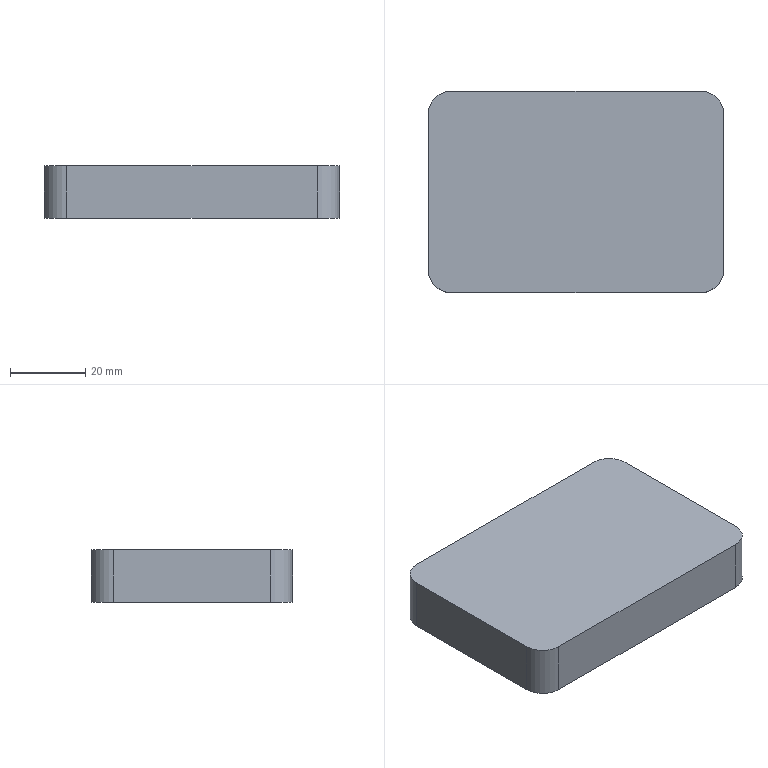Part | SolidWorks | features Extrusion 1, Fillet 1 | 1 solid | 10 faces | box 78.5 x 53.5 x 14 mm | volume 58364 mm3 | plane 6 | cylinder 4 | commonest cylinder face diameters 12 x4
STEP:
#1=CARTESIAN_POINT('',(0.,47.5,0.));
#2=VERTEX_POINT('',#1);
#3=CARTESIAN_POINT('',(0.,6.,0.));
#4=VERTEX_POINT('',#3);
#5=CARTESIAN_POINT('',(0.,0.,0.));
#6=DIRECTION('',(0.,-1.,0.));
#7=VECTOR('',#6,1000.);
#8=LINE('',#5,#7);
#9=EDGE_CURVE('',#2,#4,#8,.T.);
#10=ORIENTED_EDGE('',*,*,#9,.T.);
#11=CARTESIAN_POINT('',(0.,6.,14.));
#12=VERTEX_POINT('',#11);
#13=CARTESIAN_POINT('',(0.,6.,14.));
#14=DIRECTION('',(0.,0.,1.));
#15=VECTOR('',#14,1000.);
#16=LINE('',#13,#15);
#17=EDGE_CURVE('',#4,#12,#16,.T.);
#18=ORIENTED_EDGE('',*,*,#17,.T.);
#19=CARTESIAN_POINT('',(0.,47.5,14.));
#20=VERTEX_POINT('',#19);
#21=CARTESIAN_POINT('',(0.,0.,14.));
#22=DIRECTION('',(0.,-1.,0.));
#23=VECTOR('',#22,1000.);
#24=LINE('',#21,#23);
#25=EDGE_CURVE('',#20,#12,#24,.T.);
#26=ORIENTED_EDGE('',*,*,#25,.F.);
#27=CARTESIAN_POINT('',(0.,47.5,14.));
#28=DIRECTION('',(0.,0.,-1.));
#29=VECTOR('',#28,1000.);
#30=LINE('',#27,#29);
#31=EDGE_CURVE('',#20,#2,#30,.T.);
#32=ORIENTED_EDGE('',*,*,#31,.T.);
#33=EDGE_LOOP('',(#10,#18,#26,#32));
#34=FACE_OUTER_BOUND('',#33,.T.);
#35=CARTESIAN_POINT('',(0.,0.,14.));
#36=DIRECTION('',(1.,0.,0.));
#37=DIRECTION('',(0.,0.,-1.));
#38=AXIS2_PLACEMENT_3D('',#35,#36,#37);
#39=PLANE('',#38);
#40=ADVANCED_FACE('',(#34),#39,.F.);
#41=CARTESIAN_POINT('',(6.,0.,0.));
#42=VERTEX_POINT('',#41);
#43=CARTESIAN_POINT('',(72.5,0.,0.));
#44=VERTEX_POINT('',#43);
#45=CARTESIAN_POINT('',(0.,0.,0.));
#46=DIRECTION('',(1.,0.,0.));
#47=VECTOR('',#46,1000.);
#48=LINE('',#45,#47);
#49=EDGE_CURVE('',#42,#44,#48,.T.);
#50=ORIENTED_EDGE('',*,*,#49,.T.);
#51=CARTESIAN_POINT('',(72.5,0.,14.));
#52=VERTEX_POINT('',#51);
#53=CARTESIAN_POINT('',(72.5,0.,14.));
#54=DIRECTION('',(0.,0.,1.));
#55=VECTOR('',#54,1000.);
#56=LINE('',#53,#55);
#57=EDGE_CURVE('',#44,#52,#56,.T.);
#58=ORIENTED_EDGE('',*,*,#57,.T.);
#59=CARTESIAN_POINT('',(6.,0.,14.));
#60=VERTEX_POINT('',#59);
#61=CARTESIAN_POINT('',(0.,0.,14.));
#62=DIRECTION('',(1.,0.,0.));
#63=VECTOR('',#62,1000.);
#64=LINE('',#61,#63);
#65=EDGE_CURVE('',#60,#52,#64,.T.);
#66=ORIENTED_EDGE('',*,*,#65,.F.);
#67=CARTESIAN_POINT('',(6.,0.,14.));
#68=DIRECTION('',(0.,0.,-1.));
#69=VECTOR('',#68,1000.);
#70=LINE('',#67,#69);
#71=EDGE_CURVE('',#60,#42,#70,.T.);
#72=ORIENTED_EDGE('',*,*,#71,.T.);
#73=EDGE_LOOP('',(#50,#58,#66,#72));
#74=FACE_OUTER_BOUND('',#73,.T.);
#75=CARTESIAN_POINT('',(0.,0.,14.));
#76=DIRECTION('',(0.,1.,0.));
#77=DIRECTION('',(0.,0.,1.));
#78=AXIS2_PLACEMENT_3D('',#75,#76,#77);
#79=PLANE('',#78);
#80=ADVANCED_FACE('',(#74),#79,.F.);
#81=CARTESIAN_POINT('',(78.5,6.,0.));
#82=VERTEX_POINT('',#81);
#83=CARTESIAN_POINT('',(78.5,47.5,0.));
#84=VERTEX_POINT('',#83);
#85=CARTESIAN_POINT('',(78.5,0.,0.));
#86=DIRECTION('',(0.,1.,0.));
#87=VECTOR('',#86,1000.);
#88=LINE('',#85,#87);
#89=EDGE_CURVE('',#82,#84,#88,.T.);
#90=ORIENTED_EDGE('',*,*,#89,.T.);
#91=CARTESIAN_POINT('',(78.5,47.5,14.));
#92=VERTEX_POINT('',#91);
#93=CARTESIAN_POINT('',(78.5,47.5,14.));
#94=DIRECTION('',(0.,0.,1.));
#95=VECTOR('',#94,1000.);
#96=LINE('',#93,#95);
#97=EDGE_CURVE('',#84,#92,#96,.T.);
#98=ORIENTED_EDGE('',*,*,#97,.T.);
#99=CARTESIAN_POINT('',(78.5,6.,14.));
#100=VERTEX_POINT('',#99);
#101=CARTESIAN_POINT('',(78.5,0.,14.));
#102=DIRECTION('',(0.,1.,0.));
#103=VECTOR('',#102,1000.);
#104=LINE('',#101,#103);
#105=EDGE_CURVE('',#100,#92,#104,.T.);
#106=ORIENTED_EDGE('',*,*,#105,.F.);
#107=CARTESIAN_POINT('',(78.5,6.,14.));
#108=DIRECTION('',(0.,0.,-1.));
#109=VECTOR('',#108,1000.);
#110=LINE('',#107,#109);
#111=EDGE_CURVE('',#100,#82,#110,.T.);
#112=ORIENTED_EDGE('',*,*,#111,.T.);
#113=EDGE_LOOP('',(#90,#98,#106,#112));
#114=FACE_OUTER_BOUND('',#113,.T.);
#115=CARTESIAN_POINT('',(78.5,0.,14.));
#116=DIRECTION('',(-1.,0.,0.));
#117=DIRECTION('',(0.,0.,1.));
#118=AXIS2_PLACEMENT_3D('',#115,#116,#117);
#119=PLANE('',#118);
#120=ADVANCED_FACE('',(#114),#119,.F.);
#121=CARTESIAN_POINT('',(72.5,53.5,14.));
#122=VERTEX_POINT('',#121);
#123=CARTESIAN_POINT('',(6.,53.5,14.));
#124=VERTEX_POINT('',#123);
#125=CARTESIAN_POINT('',(0.,53.5,14.));
#126=DIRECTION('',(-1.,0.,0.));
#127=VECTOR('',#126,1000.);
#128=LINE('',#125,#127);
#129=EDGE_CURVE('',#122,#124,#128,.T.);
#130=ORIENTED_EDGE('',*,*,#129,.F.);
#131=CARTESIAN_POINT('',(72.5,53.5,0.));
#132=VERTEX_POINT('',#131);
#133=CARTESIAN_POINT('',(72.5,53.5,14.));
#134=DIRECTION('',(0.,0.,-1.));
#135=VECTOR('',#134,1000.);
#136=LINE('',#133,#135);
#137=EDGE_CURVE('',#122,#132,#136,.T.);
#138=ORIENTED_EDGE('',*,*,#137,.T.);
#139=CARTESIAN_POINT('',(6.,53.5,0.));
#140=VERTEX_POINT('',#139);
#141=CARTESIAN_POINT('',(0.,53.5,0.));
#142=DIRECTION('',(-1.,0.,0.));
#143=VECTOR('',#142,1000.);
#144=LINE('',#141,#143);
#145=EDGE_CURVE('',#132,#140,#144,.T.);
#146=ORIENTED_EDGE('',*,*,#145,.T.);
#147=CARTESIAN_POINT('',(6.,53.5,14.));
#148=DIRECTION('',(0.,0.,1.));
#149=VECTOR('',#148,1000.);
#150=LINE('',#147,#149);
#151=EDGE_CURVE('',#140,#124,#150,.T.);
#152=ORIENTED_EDGE('',*,*,#151,.T.);
#153=EDGE_LOOP('',(#130,#138,#146,#152));
#154=FACE_OUTER_BOUND('',#153,.T.);
#155=CARTESIAN_POINT('',(0.,53.5,14.));
#156=DIRECTION('',(0.,-1.,0.));
#157=DIRECTION('',(0.,0.,-1.));
#158=AXIS2_PLACEMENT_3D('',#155,#156,#157);
#159=PLANE('',#158);
#160=ADVANCED_FACE('',(#154),#159,.F.);
#161=ORIENTED_EDGE('',*,*,#105,.T.);
#162=CARTESIAN_POINT('',(72.5,47.5,14.));
#163=DIRECTION('',(0.,0.,1.));
#164=DIRECTION('',(-1.,0.,0.));
#165=AXIS2_PLACEMENT_3D('',#162,#163,#164);
#166=CIRCLE('',#165,6.);
#167=EDGE_CURVE('',#92,#122,#166,.T.);
#168=ORIENTED_EDGE('',*,*,#167,.T.);
#169=ORIENTED_EDGE('',*,*,#129,.T.);
#170=CARTESIAN_POINT('',(6.,47.5,14.));
#171=DIRECTION('',(0.,0.,1.));
#172=DIRECTION('',(-1.,0.,0.));
#173=AXIS2_PLACEMENT_3D('',#170,#171,#172);
#174=CIRCLE('',#173,6.);
#175=EDGE_CURVE('',#124,#20,#174,.T.);
#176=ORIENTED_EDGE('',*,*,#175,.T.);
#177=ORIENTED_EDGE('',*,*,#25,.T.);
#178=CARTESIAN_POINT('',(6.,6.,14.));
#179=DIRECTION('',(0.,0.,1.));
#180=DIRECTION('',(-1.,0.,0.));
#181=AXIS2_PLACEMENT_3D('',#178,#179,#180);
#182=CIRCLE('',#181,6.);
#183=EDGE_CURVE('',#12,#60,#182,.T.);
#184=ORIENTED_EDGE('',*,*,#183,.T.);
#185=ORIENTED_EDGE('',*,*,#65,.T.);
#186=CARTESIAN_POINT('',(72.5,6.,14.));
#187=DIRECTION('',(0.,0.,1.));
#188=DIRECTION('',(-1.,0.,0.));
#189=AXIS2_PLACEMENT_3D('',#186,#187,#188);
#190=CIRCLE('',#189,6.);
#191=EDGE_CURVE('',#52,#100,#190,.T.);
#192=ORIENTED_EDGE('',*,*,#191,.T.);
#193=EDGE_LOOP('',(#161,#168,#169,#176,#177,#184,#185,#192));
#194=FACE_OUTER_BOUND('',#193,.T.);
#195=CARTESIAN_POINT('',(0.,0.,14.));
#196=DIRECTION('',(0.,0.,-1.));
#197=DIRECTION('',(-1.,0.,0.));
#198=AXIS2_PLACEMENT_3D('',#195,#196,#197);
#199=PLANE('',#198);
#200=ADVANCED_FACE('',(#194),#199,.F.);
#201=ORIENTED_EDGE('',*,*,#145,.F.);
#202=CARTESIAN_POINT('',(72.5,47.5,0.));
#203=DIRECTION('',(0.,0.,-1.));
#204=DIRECTION('',(-1.,0.,0.));
#205=AXIS2_PLACEMENT_3D('',#202,#203,#204);
#206=CIRCLE('',#205,6.);
#207=EDGE_CURVE('',#132,#84,#206,.T.);
#208=ORIENTED_EDGE('',*,*,#207,.T.);
#209=ORIENTED_EDGE('',*,*,#89,.F.);
#210=CARTESIAN_POINT('',(72.5,6.,0.));
#211=DIRECTION('',(0.,0.,-1.));
#212=DIRECTION('',(-1.,0.,0.));
#213=AXIS2_PLACEMENT_3D('',#210,#211,#212);
#214=CIRCLE('',#213,6.);
#215=EDGE_CURVE('',#82,#44,#214,.T.);
#216=ORIENTED_EDGE('',*,*,#215,.T.);
#217=ORIENTED_EDGE('',*,*,#49,.F.);
#218=CARTESIAN_POINT('',(6.,6.,0.));
#219=DIRECTION('',(0.,0.,-1.));
#220=DIRECTION('',(-1.,0.,0.));
#221=AXIS2_PLACEMENT_3D('',#218,#219,#220);
#222=CIRCLE('',#221,6.);
#223=EDGE_CURVE('',#42,#4,#222,.T.);
#224=ORIENTED_EDGE('',*,*,#223,.T.);
#225=ORIENTED_EDGE('',*,*,#9,.F.);
#226=CARTESIAN_POINT('',(6.,47.5,0.));
#227=DIRECTION('',(0.,0.,-1.));
#228=DIRECTION('',(-1.,0.,0.));
#229=AXIS2_PLACEMENT_3D('',#226,#227,#228);
#230=CIRCLE('',#229,6.);
#231=EDGE_CURVE('',#2,#140,#230,.T.);
#232=ORIENTED_EDGE('',*,*,#231,.T.);
#233=EDGE_LOOP('',(#201,#208,#209,#216,#217,#224,#225,#232));
#234=FACE_OUTER_BOUND('',#233,.T.);
#235=CARTESIAN_POINT('',(0.,0.,0.));
#236=DIRECTION('',(0.,0.,-1.));
#237=DIRECTION('',(-1.,0.,0.));
#238=AXIS2_PLACEMENT_3D('',#235,#236,#237);
#239=PLANE('',#238);
#240=ADVANCED_FACE('',(#234),#239,.T.);
#241=ORIENTED_EDGE('',*,*,#167,.F.);
#242=ORIENTED_EDGE('',*,*,#97,.F.);
#243=ORIENTED_EDGE('',*,*,#207,.F.);
#244=ORIENTED_EDGE('',*,*,#137,.F.);
#245=EDGE_LOOP('',(#241,#242,#243,#244));
#246=FACE_OUTER_BOUND('',#245,.T.);
#247=CARTESIAN_POINT('',(72.5,47.5,14.));
#248=DIRECTION('',(0.,0.,-1.));
#249=DIRECTION('',(-1.,0.,0.));
#250=AXIS2_PLACEMENT_3D('',#247,#248,#249);
#251=CYLINDRICAL_SURFACE('',#250,6.);
#252=ADVANCED_FACE('',(#246),#251,.T.);
#253=ORIENTED_EDGE('',*,*,#191,.F.);
#254=ORIENTED_EDGE('',*,*,#57,.F.);
#255=ORIENTED_EDGE('',*,*,#215,.F.);
#256=ORIENTED_EDGE('',*,*,#111,.F.);
#257=EDGE_LOOP('',(#253,#254,#255,#256));
#258=FACE_OUTER_BOUND('',#257,.T.);
#259=CARTESIAN_POINT('',(72.5,6.,14.));
#260=DIRECTION('',(0.,0.,-1.));
#261=DIRECTION('',(-1.,0.,0.));
#262=AXIS2_PLACEMENT_3D('',#259,#260,#261);
#263=CYLINDRICAL_SURFACE('',#262,6.);
#264=ADVANCED_FACE('',(#258),#263,.T.);
#265=ORIENTED_EDGE('',*,*,#183,.F.);
#266=ORIENTED_EDGE('',*,*,#17,.F.);
#267=ORIENTED_EDGE('',*,*,#223,.F.);
#268=ORIENTED_EDGE('',*,*,#71,.F.);
#269=EDGE_LOOP('',(#265,#266,#267,#268));
#270=FACE_OUTER_BOUND('',#269,.T.);
#271=CARTESIAN_POINT('',(6.,6.,14.));
#272=DIRECTION('',(0.,0.,-1.));
#273=DIRECTION('',(-1.,0.,0.));
#274=AXIS2_PLACEMENT_3D('',#271,#272,#273);
#275=CYLINDRICAL_SURFACE('',#274,6.);
#276=ADVANCED_FACE('',(#270),#275,.T.);
#277=ORIENTED_EDGE('',*,*,#175,.F.);
#278=ORIENTED_EDGE('',*,*,#151,.F.);
#279=ORIENTED_EDGE('',*,*,#231,.F.);
#280=ORIENTED_EDGE('',*,*,#31,.F.);
#281=EDGE_LOOP('',(#277,#278,#279,#280));
#282=FACE_OUTER_BOUND('',#281,.T.);
#283=CARTESIAN_POINT('',(6.,47.5,14.));
#284=DIRECTION('',(0.,0.,-1.));
#285=DIRECTION('',(-1.,0.,0.));
#286=AXIS2_PLACEMENT_3D('',#283,#284,#285);
#287=CYLINDRICAL_SURFACE('',#286,6.);
#288=ADVANCED_FACE('',(#282),#287,.T.);
#289=CLOSED_SHELL('',(#40,#80,#120,#160,#200,#240,#252,#264,#276,#288));
#290=MANIFOLD_SOLID_BREP('',#289);
#291=CARTESIAN_POINT('',(0.,0.,0.));
#292=DIRECTION('',(0.,0.,1.));
#293=DIRECTION('',(1.,0.,0.));
#294=AXIS2_PLACEMENT_3D('',#291,#292,#293);
#295=(LENGTH_UNIT()NAMED_UNIT(*)SI_UNIT(.MILLI.,.METRE.));
#296=UNCERTAINTY_MEASURE_WITH_UNIT(LENGTH_MEASURE(0.00001),#295,'','');
#297=(NAMED_UNIT(*)PLANE_ANGLE_UNIT()SI_UNIT($,.RADIAN.));
#298=(NAMED_UNIT(*)SI_UNIT($,.STERADIAN.)SOLID_ANGLE_UNIT());
#299=(GEOMETRIC_REPRESENTATION_CONTEXT(3)GLOBAL_UNCERTAINTY_ASSIGNED_CONTEXT((#296))GLOBAL_UNIT_ASSIGNED_CONTEXT((#295,#297,#298))REPRESENTATION_CONTEXT('',''));
#300=ADVANCED_BREP_SHAPE_REPRESENTATION('',(#290,#294),#299);